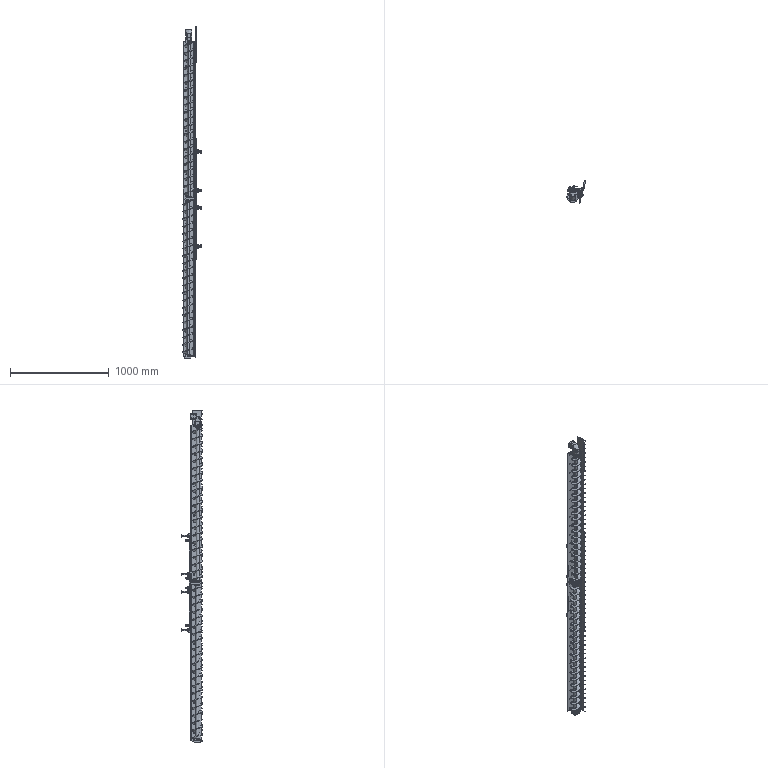Part | 74 solids | 3704 faces | volume 10529066 mm3 | cylinder 1776 | plane 1546 | cone 185 | torus 132 | spline 57 | sphere 8 | commonest cylinder face diameters 4.2 x414 4 x114 6 x107 5 x101 5.8 x78 5.5 x72